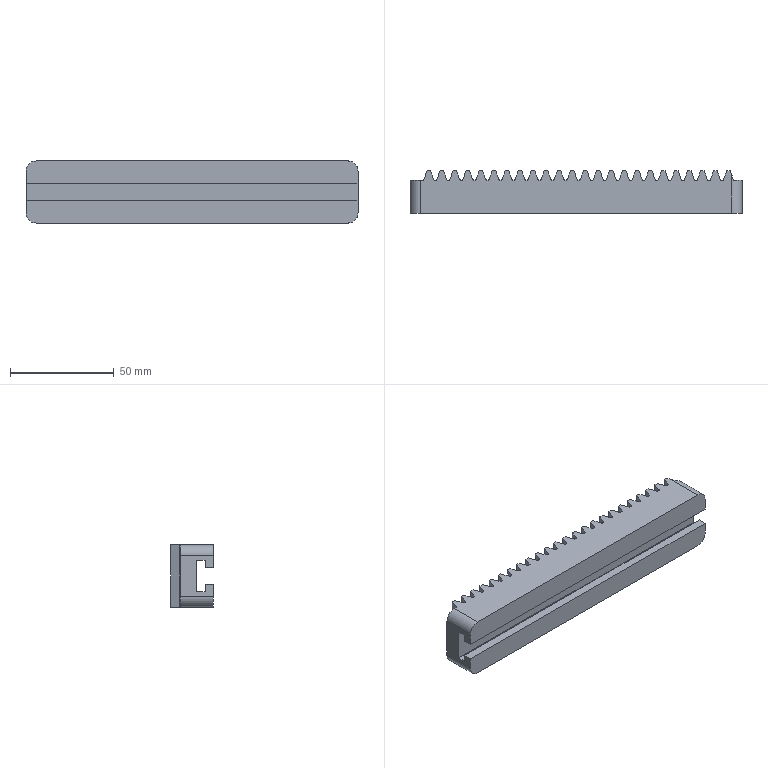Part | STEP file | RACK2_id430_x_t | 1 solid | 162 faces | box 160 x 20.596 x 30 mm | volume 72119 mm3 | plane 110 | cylinder 52 | commonest cylinder face diameters 1 x48 10 x4